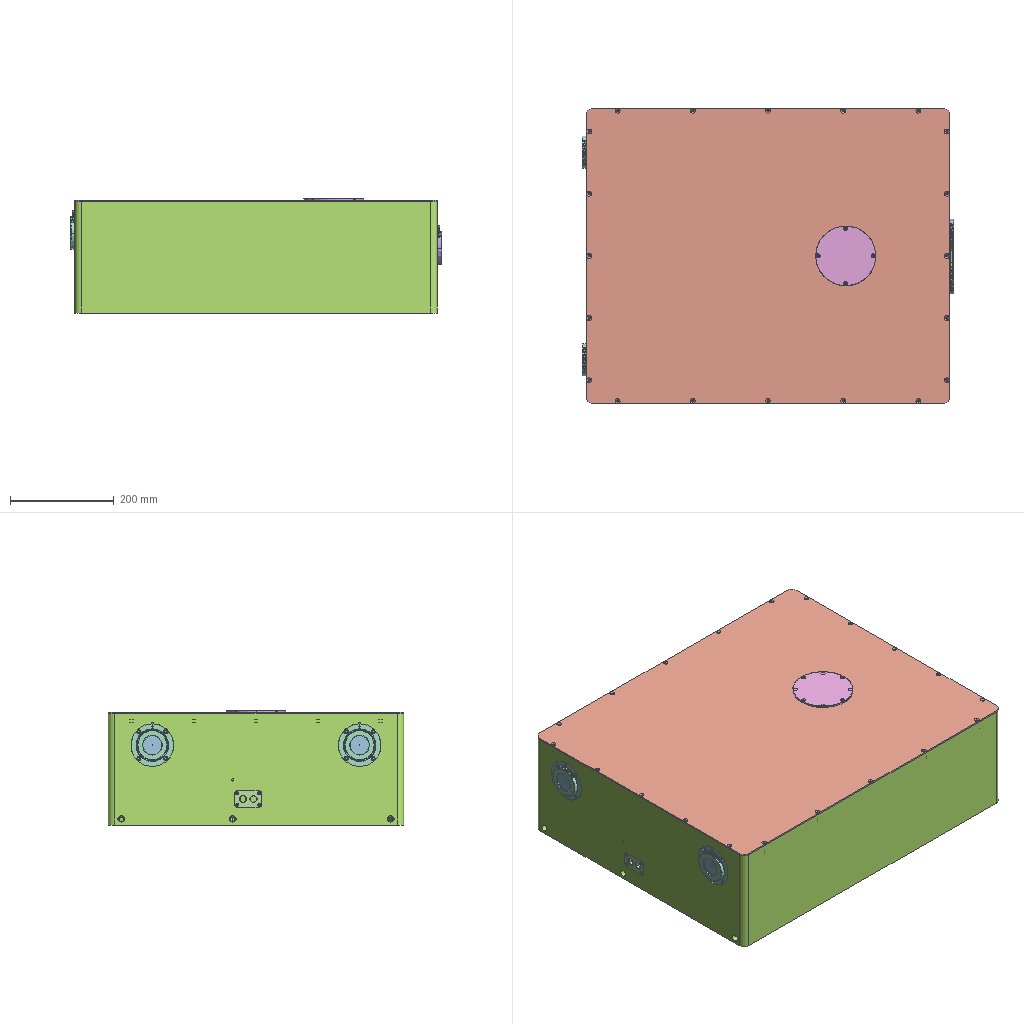Assembly | SolidWorks | 24 different items | 67 placed | box 717 x 570 x 222 mm
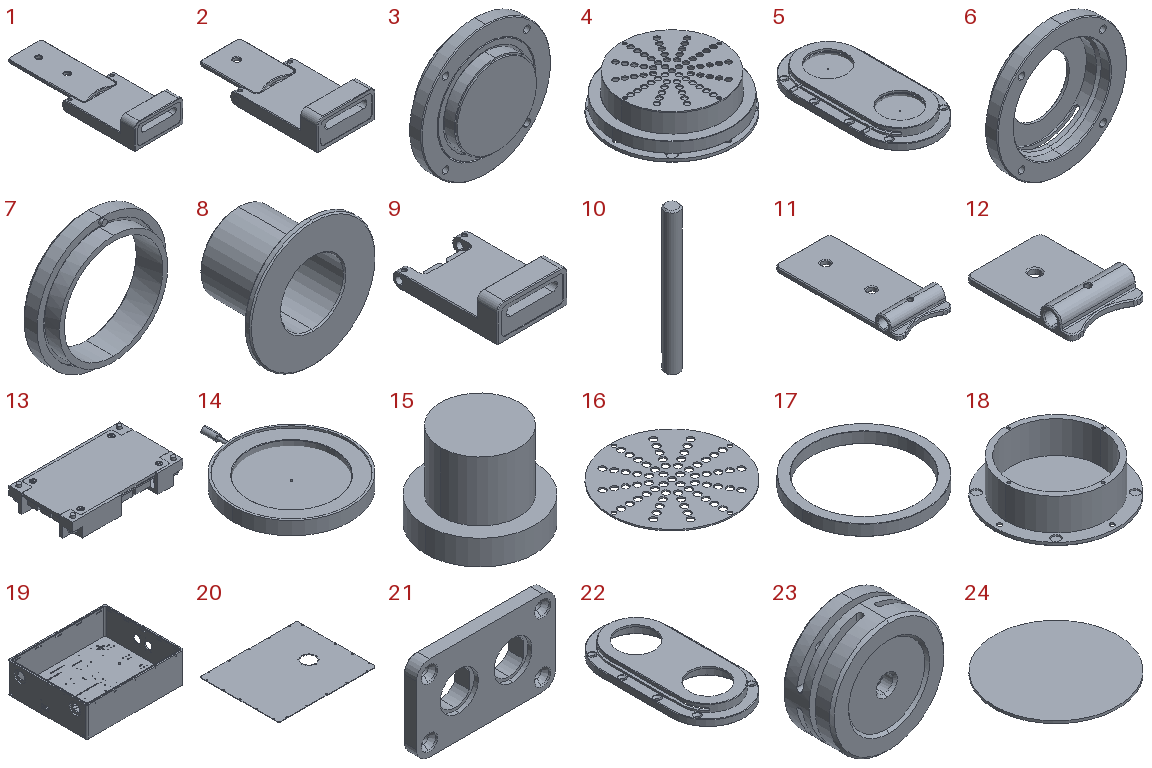Parts list (item | name | quantity | parent item | size | volume | features):
1 | (subassembly) | x2 | - | 50 x 138.5 x 25 mm | 43110 mm3 | -
2 | (subassembly) | x4 | - | 50 x 109.5 x 25 mm | 40151 mm3 | -
3 | (subassembly) | x2 | - | 82.5 x 22.992 x 84.25 mm | 44307 mm3 | -
4 | (subassembly) | x1 | - | 116 x 116 x 34 mm | 105330 mm3 | features InContextFeatHolder 2, RefAxis 1
5 | (subassembly) | x1 | - | 84.25 x 164.5 x 22 mm | 108693 mm3 | -
6 | - | x2 | in 3 | 82.5 x 16 x 82.5 mm | 23486 mm3 | features MoveFace 2, Chamfer 1, Fillet 1, HoleWzd 1, ICE 1, Revolution 1
7 | - | x4 | in 3, 5 | 61 x 13.5 x 61 mm | 10536 mm3 | features Chamfer 2, ICE 2, Revolution 1
8 | - | x12 | in 1, 2 | 10 x 6 x 10 mm | 76.5 mm3 | features Chamfer 1, Revolution 1
9 | - | x6 | in 1, 2 | 50 x 75 x 25 mm | 33141 mm3 | features ICE 6, Chamfer 2, Fillet 2, Extrusion 1, HoleWzd 1, MoveFace 1
10 | - | x6 | in 1, 2 | 5 x 5 x 50 mm | 969.137 mm3 | features Chamfer 1, Extrusion 1, ICE 1
11 | - | x2 | in 1 | 34.9 x 78.5 x 10 mm | 8847 mm3 | features MoveFace 4, Fillet 2, 3DProfileFeature 1, Chamfer 1, Extrusion 1, HoleWzd 1, ICE 1
12 | - | x4 | in 2 | 34.9 x 49.5 x 10 mm | 5888 mm3 | features MoveFace 4, Fillet 2, 3DProfileFeature 1, Chamfer 1, DelFace 1, Extrusion 1, HoleWzd 1, ICE 1
13 | - | x2 | - | 90 x 52 x 16.8 mm | 31722 mm3 | features BaseBody 28
14 | - | x4 | in 3, 5 | 58 x 72 x 6.5 mm | 8321 mm3 | features ICE 3, Chamfer 1, Extrusion 1, MoveFace 1, Revolution 1
15 | - | x3 | - | 21.9 x 21.9 x 17 mm | 3945 mm3 | features ICE 2, Extrusion 1
16 | - | x1 | in 4 | 94.5 x 94.5 x 1 mm | 5705 mm3 | features Cut 2, Extrusion 1
17 | - | x1 | in 4 | 112 x 112 x 10 mm | 26527 mm3 | features Chamfer 1, Extrusion 1, HoleWzd 1, ICE 1
18 | - | x1 | in 4 | 116 x 116 x 33 mm | 73097 mm3 | features HoleWzd 2, ICE 2, Chamfer 1, Extrusion 1
19 | - | x1 | - | 700 x 570 x 215 mm | 18356109 mm3 | features HoleWzd 21, Cut 16, ICE 8, MoveFace 6, Fillet 3, CutThin 2, Chamfer 1, Extrusion 1, Shell 1
20 | - | x1 | - | 700 x 570 x 3 mm | 1172283 mm3 | features Cut 2, Extrusion 1, HoleWzd 1, ICE 1
21 | - | x1 | - | 51.6 x 7 x 31.6 mm | 7439 mm3 | features ICE 3, Chamfer 1, Extrusion 1, Fillet 1, HoleWzd 1
22 | - | x1 | in 5 | 82.5 x 164.5 x 16 mm | 70978 mm3 | features ICE 5, Chamfer 2, HoleWzd 2, Cut 1, Extrusion 1, Fillet 1, MoveFace 1
23 | - | x3 | - | 48 x 21 x 48 mm | 20684 mm3 | features ICE 3, Chamfer 1, Extrusion 1, HoleWzd 1
24 | - | x2 | in 3 | 50 x 50 x 1 mm | 1963 mm3 | features Extrusion 1
Mates (type | each side: item.copy, entity, surface, feature):
In the top assembly
Concentric | 19.1 face cylinder Cut-Extrude 1 | 6.1 face cylinder Revolve 1
Parallel | 19.1 face plane Boss-Extrude 1 | 3.1 plane
Coincident | 19.1 face plane Cut-Extrude 1 | 6.2 face plane Revolve 1
Concentric | 19.1 face cylinder Cut-Extrude 1 | 6.2 face cylinder Revolve 1
Coincident | 19.1 face plane Boss-Extrude 1 | 6.1 face plane Revolve 1
Concentric | 19.1 face cylinder Cut-Extrude 7 | 22.1 face cylinder Boss-Extrude 1
Coincident | 19.1 face plane Cut-Extrude 16 | 23.1 face plane Boss-Extrude 1
Concentric | 19.1 face cylinder Cut-Extrude 16 | 23.2 face cylinder Boss-Extrude 1
Coincident | 23.1 face plane Boss-Extrude 1 | 23.2 face plane Boss-Extrude 1
Concentric | 19.1 face cylinder Cut-Extrude 15 | 23.2 face cylinder M4 Tapped Hole 1
Concentric | 19.1 face cylinder Cut-Extrude 16 | 23.3 face cylinder Boss-Extrude 1
Coincident | 23.2 face plane Boss-Extrude 1 | 23.3 face plane Boss-Extrude 1
Concentric | 19.1 face cylinder Cut-Extrude 15 | 23.3 face cylinder M4 Tapped Hole 1
Coincident | 19.1 face plane Boss-Extrude 1 | 20.1 face plane Boss-Extrude 1 | 3 times
Parallel | 19.1 face plane Boss-Extrude 1 | 4.1 plane
Coincident | 19.1 face plane Cut-Extrude 13 | 15.1 face plane Boss-Extrude 1
Concentric | 19.1 face cylinder Cut-Extrude 12 | 15.1 face cylinder Boss-Extrude 1
Concentric | 19.1 face cylinder Cut-Extrude 16 | 23.1 face cylinder Boss-Extrude 1
Concentric | 19.1 face cylinder Cut-Extrude 12 | 15.2 face cylinder Boss-Extrude 2
Coincident | 15.1 face plane Boss-Extrude 1 | 15.2 face plane Boss-Extrude 1
Concentric | 19.1 face cylinder Cut-Extrude 12 | 15.3 face cylinder Boss-Extrude 2
Coincident | 15.1 face plane Boss-Extrude 1 | 15.3 face plane Boss-Extrude 1
Coincident | 19.1 face plane Shell 1 | 9.1 face plane Boss-Extrude 1
DistanceDim | 19.1 face plane Shell 1 | 9.1 face plane Boss-Extrude 1
DistanceDim | 12.1 face cylinder Boss-Extrude 2 | 19.1 face plane Shell 1
Coincident | 19.1 face plane Shell 1 | 9.2 face plane Boss-Extrude 1
DistanceDim | 12.2 face cylinder Boss-Extrude 2 | 19.1 face plane Shell 1
DistanceDim | 9.2 face plane Boss-Extrude 1 | 19.1 face plane Shell 1
Coincident | 19.1 face plane Shell 1 | 9.3 face plane Boss-Extrude 1
Coincident | 19.1 face plane Shell 1 | 9.4 face plane Boss-Extrude 1
Coincident | 19.1 face plane Shell 1 | 9.5 face plane Boss-Extrude 1
Coincident | 19.1 face plane Shell 1 | 9.6 face plane Boss-Extrude 1
In subassembly 2
Coincident | 9.7 face plane Cut-Extrude 3 | 8.1 face plane Revolve 1
Coincident | 9.7 face plane Cut-Extrude 3 | 8.2 face plane Revolve 1
Concentric | 10.1 face cylinder Boss-Extrude 1 | 8.2 face cylinder Revolve 1
Concentric | 12.3 face cylinder Boss-Extrude 1 | 10.1 face cylinder Boss-Extrude 1
DistanceDim | 8.1 face plane Revolve 1 | 12.3 face plane Boss-Extrude 1
Coincident | 9.7 face plane Boss-Extrude 1 | 10.1 face plane Boss-Extrude 1
Parallel | 9.7 face plane Boss-Extrude 1 | 10.1 face plane Cut-Extrude 1
Concentric | 9.7 face cylinder Cut-Extrude 6 | 10.1 face cylinder Boss-Extrude 1
Parallel | 9.7 face plane Boss-Extrude 1 | 12.3 face plane Boss-Extrude 1
In subassembly 1
Coincident | 9.7 face plane Cut-Extrude 3 | 8.1 face plane Revolve 1
Coincident | 9.7 face plane Cut-Extrude 3 | 8.2 face plane Revolve 1
Concentric | 10.1 face cylinder Boss-Extrude 1 | 8.2 face cylinder Revolve 1
Concentric | 11.1 face cylinder Boss-Extrude 1 | 10.1 face cylinder Boss-Extrude 1
DistanceDim | 8.1 face plane Revolve 1 | 11.1 face plane Boss-Extrude 1
Coincident | 9.7 face plane Boss-Extrude 1 | 10.1 face plane Boss-Extrude 1
Parallel | 9.7 face plane Boss-Extrude 1 | 10.1 face plane Cut-Extrude 1
In subassembly 3
Coincident | 6.3 face plane Revolve 1 | 14.1 face plane Boss-Extrude 1
Concentric | 6.3 face cylinder Revolve 1 | 14.1 face cylinder Boss-Extrude 1
Coincident | 7.1 face plane Revolve 1 | 14.1 face plane Boss-Extrude 1
PlanarAngleDim | 7.1 plane | 3.2 plane
Coincident | 7.1 face plane Cut-Extrude 1 | 24.1 face plane Boss-Extrude 1
Concentric | 7.1 face cylinder Revolve 1 | 6.3 face cylinder Revolve 1
In subassembly 5
Coincident | 22.2 face plane Cut-Extrude 2 | 14.1 face plane Boss-Extrude 1
Concentric | 22.2 face cylinder Cut-Extrude 2 | 14.1 face cylinder Boss-Extrude 1
Parallel | 22.2 face plane Boss-Extrude 1 | 14.1 plane
Coincident | 14.1 face plane Boss-Extrude 2 | 14.2 face plane Boss-Extrude 2 | 2 times
Concentric | 22.2 face cylinder Cut-Extrude 3 | 14.2 face cylinder Boss-Extrude 1
Coincident | 14.1 face plane Boss-Extrude 1 | 7.1 face plane Revolve 1
Concentric | 22.2 face cylinder Cut-Extrude 3 | 7.1 face cylinder Revolve 1
Concentric | 22.2 face cylinder Cut-Extrude 3 | 7.2 face cylinder Revolve 1
Coincident | 14.2 face plane Boss-Extrude 1 | 7.2 face plane Revolve 1
Parallel | 22.2 face plane Boss-Extrude 1 | 7.2 plane
Parallel | 22.2 face plane Boss-Extrude 1 | 7.1 plane
In subassembly 4
Coincident | 18.1 face plane Boss-Extrude 2 | 16.1 face plane Boss-Extrude 1
Concentric | 18.1 face cylinder Boss-Extrude 2 | 16.1 face cylinder Boss-Extrude 1